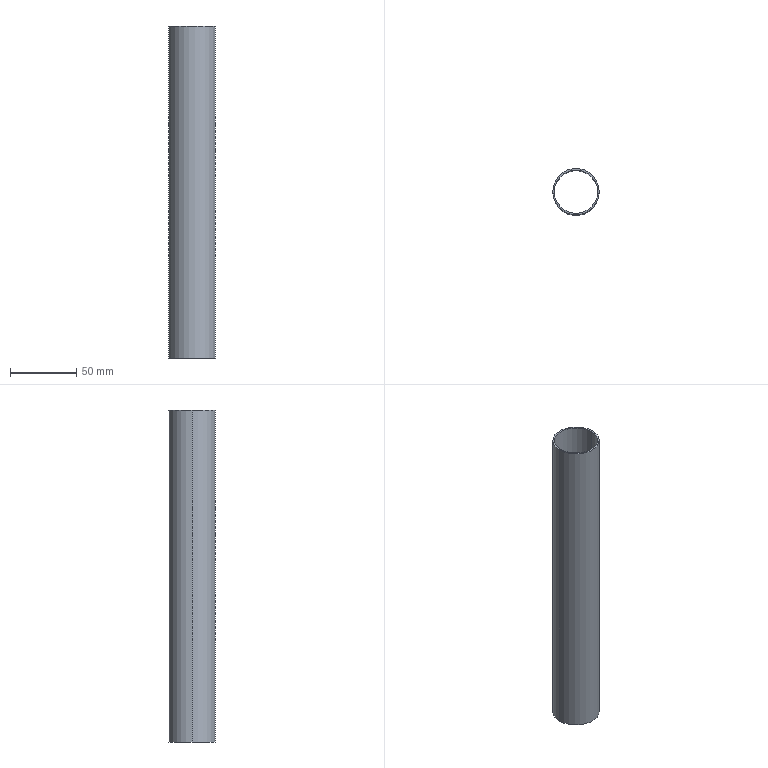Part | STEP file | copper tube 41 | 1 solid | 6 faces | box 35 x 35 x 250 mm | volume 31856 mm3 | cylinder 4 | plane 2 | commonest cylinder face diameters 32.6 x2 35 x2
STEP:
#1=CARTESIAN_POINT('',(0.,0.,0.));
#2=DIRECTION('',(0.,0.,1.));
#3=DIRECTION('',(1.,0.,0.));
#4=AXIS2_PLACEMENT_3D('',#1,#2,#3);
#5=CARTESIAN_POINT('',(16.3,0.,-5.));
#6=VERTEX_POINT('',#5);
#7=CARTESIAN_POINT('',(16.3,0.,245.));
#8=VERTEX_POINT('',#7);
#9=CARTESIAN_POINT('',(16.3,0.,-5.));
#10=DIRECTION('',(0.,0.,1.));
#11=VECTOR('',#10,1.);
#12=LINE('',#9,#11);
#13=CARTESIAN_POINT('',(0.,0.,-5.));
#14=DIRECTION('',(0.,0.,1.));
#15=DIRECTION('',(1.,0.,0.));
#16=AXIS2_PLACEMENT_3D('',#13,#14,#15);
#17=CYLINDRICAL_SURFACE('',#16,16.3);
#18=CARTESIAN_POINT('',(6.283,0.));
#19=DIRECTION('',(0.,1.));
#20=VECTOR('',#19,1.);
#21=LINE('',#18,#20);
#22=(GEOMETRIC_REPRESENTATION_CONTEXT(2)PARAMETRIC_REPRESENTATION_CONTEXT()REPRESENTATION_CONTEXT('',''));
#23=DEFINITIONAL_REPRESENTATION('',(#21),#22);
#24=PCURVE('',#17,#23);
#25=CARTESIAN_POINT('',(0.,0.,-5.));
#26=DIRECTION('',(0.,0.,1.));
#27=DIRECTION('',(1.,0.,0.));
#28=AXIS2_PLACEMENT_3D('',#25,#26,#27);
#29=CYLINDRICAL_SURFACE('',#28,16.3);
#30=CARTESIAN_POINT('',(0.,0.));
#31=DIRECTION('',(0.,1.));
#32=VECTOR('',#31,1.);
#33=LINE('',#30,#32);
#34=(GEOMETRIC_REPRESENTATION_CONTEXT(2)PARAMETRIC_REPRESENTATION_CONTEXT()REPRESENTATION_CONTEXT('',''));
#35=DEFINITIONAL_REPRESENTATION('',(#33),#34);
#36=PCURVE('',#29,#35);
#37=SURFACE_CURVE('',#12,(#24,#36),.PCURVE_S1.);
#38=EDGE_CURVE('',#6,#8,#37,.T.);
#39=ORIENTED_EDGE('',*,*,#38,.T.);
#40=CARTESIAN_POINT('',(-16.3,0.,245.));
#41=VERTEX_POINT('',#40);
#42=CARTESIAN_POINT('',(0.,0.,245.));
#43=DIRECTION('',(0.,0.,1.));
#44=DIRECTION('',(1.,0.,0.));
#45=AXIS2_PLACEMENT_3D('',#42,#43,#44);
#46=CIRCLE('',#45,16.3);
#47=CARTESIAN_POINT('',(0.,250.));
#48=DIRECTION('',(1.,0.));
#49=VECTOR('',#48,1.);
#50=LINE('',#47,#49);
#51=(GEOMETRIC_REPRESENTATION_CONTEXT(2)PARAMETRIC_REPRESENTATION_CONTEXT()REPRESENTATION_CONTEXT('',''));
#52=DEFINITIONAL_REPRESENTATION('',(#50),#51);
#53=PCURVE('',#17,#52);
#54=CARTESIAN_POINT('',(0.,0.,245.));
#55=DIRECTION('',(0.,0.,1.));
#56=DIRECTION('',(1.,0.,0.));
#57=AXIS2_PLACEMENT_3D('',#54,#55,#56);
#58=PLANE('',#57);
#59=CARTESIAN_POINT('',(0.,0.));
#60=DIRECTION('',(1.,0.));
#61=AXIS2_PLACEMENT_2D('',#59,#60);
#62=CIRCLE('',#61,16.3);
#63=(GEOMETRIC_REPRESENTATION_CONTEXT(2)PARAMETRIC_REPRESENTATION_CONTEXT()REPRESENTATION_CONTEXT('',''));
#64=DEFINITIONAL_REPRESENTATION('',(#62),#63);
#65=PCURVE('',#58,#64);
#66=SURFACE_CURVE('',#46,(#53,#65),.PCURVE_S1.);
#67=EDGE_CURVE('',#41,#8,#66,.T.);
#68=ORIENTED_EDGE('',*,*,#67,.F.);
#69=CARTESIAN_POINT('',(-16.3,0.,-5.));
#70=VERTEX_POINT('',#69);
#71=CARTESIAN_POINT('',(-16.3,0.,-5.));
#72=DIRECTION('',(0.,0.,1.));
#73=VECTOR('',#72,1.);
#74=LINE('',#71,#73);
#75=CARTESIAN_POINT('',(3.142,0.));
#76=DIRECTION('',(0.,1.));
#77=VECTOR('',#76,1.);
#78=LINE('',#75,#77);
#79=(GEOMETRIC_REPRESENTATION_CONTEXT(2)PARAMETRIC_REPRESENTATION_CONTEXT()REPRESENTATION_CONTEXT('',''));
#80=DEFINITIONAL_REPRESENTATION('',(#78),#79);
#81=PCURVE('',#17,#80);
#82=CARTESIAN_POINT('',(3.142,0.));
#83=DIRECTION('',(0.,1.));
#84=VECTOR('',#83,1.);
#85=LINE('',#82,#84);
#86=(GEOMETRIC_REPRESENTATION_CONTEXT(2)PARAMETRIC_REPRESENTATION_CONTEXT()REPRESENTATION_CONTEXT('',''));
#87=DEFINITIONAL_REPRESENTATION('',(#85),#86);
#88=PCURVE('',#29,#87);
#89=SURFACE_CURVE('',#74,(#81,#88),.PCURVE_S1.);
#90=EDGE_CURVE('',#70,#41,#89,.T.);
#91=ORIENTED_EDGE('',*,*,#90,.F.);
#92=CARTESIAN_POINT('',(0.,0.,-5.));
#93=DIRECTION('',(0.,0.,1.));
#94=DIRECTION('',(1.,0.,0.));
#95=AXIS2_PLACEMENT_3D('',#92,#93,#94);
#96=CIRCLE('',#95,16.3);
#97=CARTESIAN_POINT('',(0.,0.));
#98=DIRECTION('',(1.,0.));
#99=VECTOR('',#98,1.);
#100=LINE('',#97,#99);
#101=(GEOMETRIC_REPRESENTATION_CONTEXT(2)PARAMETRIC_REPRESENTATION_CONTEXT()REPRESENTATION_CONTEXT('',''));
#102=DEFINITIONAL_REPRESENTATION('',(#100),#101);
#103=PCURVE('',#17,#102);
#104=CARTESIAN_POINT('',(0.,0.,-5.));
#105=DIRECTION('',(0.,0.,1.));
#106=DIRECTION('',(1.,0.,0.));
#107=AXIS2_PLACEMENT_3D('',#104,#105,#106);
#108=PLANE('',#107);
#109=CARTESIAN_POINT('',(0.,0.));
#110=DIRECTION('',(1.,0.));
#111=AXIS2_PLACEMENT_2D('',#109,#110);
#112=CIRCLE('',#111,16.3);
#113=(GEOMETRIC_REPRESENTATION_CONTEXT(2)PARAMETRIC_REPRESENTATION_CONTEXT()REPRESENTATION_CONTEXT('',''));
#114=DEFINITIONAL_REPRESENTATION('',(#112),#113);
#115=PCURVE('',#108,#114);
#116=SURFACE_CURVE('',#96,(#103,#115),.PCURVE_S1.);
#117=EDGE_CURVE('',#70,#6,#116,.T.);
#118=ORIENTED_EDGE('',*,*,#117,.T.);
#119=EDGE_LOOP('',(#39,#68,#91,#118));
#120=FACE_BOUND('',#119,.F.);
#121=ADVANCED_FACE('',(#120),#17,.F.);
#122=CARTESIAN_POINT('',(17.5,0.,245.));
#123=VERTEX_POINT('',#122);
#124=CARTESIAN_POINT('',(-17.5,0.,245.));
#125=VERTEX_POINT('',#124);
#126=CARTESIAN_POINT('',(0.,0.,245.));
#127=DIRECTION('',(0.,0.,1.));
#128=DIRECTION('',(1.,0.,0.));
#129=AXIS2_PLACEMENT_3D('',#126,#127,#128);
#130=CIRCLE('',#129,17.5);
#131=CARTESIAN_POINT('',(0.,0.,245.));
#132=DIRECTION('',(0.,0.,-1.));
#133=DIRECTION('',(-1.,0.,0.));
#134=AXIS2_PLACEMENT_3D('',#131,#132,#133);
#135=CYLINDRICAL_SURFACE('',#134,17.5);
#136=CARTESIAN_POINT('',(3.142,0.));
#137=DIRECTION('',(-1.,0.));
#138=VECTOR('',#137,1.);
#139=LINE('',#136,#138);
#140=(GEOMETRIC_REPRESENTATION_CONTEXT(2)PARAMETRIC_REPRESENTATION_CONTEXT()REPRESENTATION_CONTEXT('',''));
#141=DEFINITIONAL_REPRESENTATION('',(#139),#140);
#142=PCURVE('',#135,#141);
#143=CARTESIAN_POINT('',(0.,0.));
#144=DIRECTION('',(1.,0.));
#145=AXIS2_PLACEMENT_2D('',#143,#144);
#146=CIRCLE('',#145,17.5);
#147=(GEOMETRIC_REPRESENTATION_CONTEXT(2)PARAMETRIC_REPRESENTATION_CONTEXT()REPRESENTATION_CONTEXT('',''));
#148=DEFINITIONAL_REPRESENTATION('',(#146),#147);
#149=PCURVE('',#58,#148);
#150=SURFACE_CURVE('',#130,(#142,#149),.PCURVE_S1.);
#151=EDGE_CURVE('',#123,#125,#150,.T.);
#152=ORIENTED_EDGE('',*,*,#151,.F.);
#153=CARTESIAN_POINT('',(17.5,0.,-5.));
#154=VERTEX_POINT('',#153);
#155=CARTESIAN_POINT('',(17.5,0.,245.));
#156=DIRECTION('',(0.,0.,-1.));
#157=VECTOR('',#156,1.);
#158=LINE('',#155,#157);
#159=CARTESIAN_POINT('',(3.142,0.));
#160=DIRECTION('',(0.,1.));
#161=VECTOR('',#160,1.);
#162=LINE('',#159,#161);
#163=(GEOMETRIC_REPRESENTATION_CONTEXT(2)PARAMETRIC_REPRESENTATION_CONTEXT()REPRESENTATION_CONTEXT('',''));
#164=DEFINITIONAL_REPRESENTATION('',(#162),#163);
#165=PCURVE('',#135,#164);
#166=CARTESIAN_POINT('',(0.,0.,245.));
#167=DIRECTION('',(0.,0.,-1.));
#168=DIRECTION('',(-1.,0.,0.));
#169=AXIS2_PLACEMENT_3D('',#166,#167,#168);
#170=CYLINDRICAL_SURFACE('',#169,17.5);
#171=CARTESIAN_POINT('',(3.142,0.));
#172=DIRECTION('',(0.,1.));
#173=VECTOR('',#172,1.);
#174=LINE('',#171,#173);
#175=(GEOMETRIC_REPRESENTATION_CONTEXT(2)PARAMETRIC_REPRESENTATION_CONTEXT()REPRESENTATION_CONTEXT('',''));
#176=DEFINITIONAL_REPRESENTATION('',(#174),#175);
#177=PCURVE('',#170,#176);
#178=SURFACE_CURVE('',#158,(#165,#177),.PCURVE_S1.);
#179=EDGE_CURVE('',#123,#154,#178,.T.);
#180=ORIENTED_EDGE('',*,*,#179,.T.);
#181=CARTESIAN_POINT('',(-17.5,0.,-5.));
#182=VERTEX_POINT('',#181);
#183=CARTESIAN_POINT('',(0.,0.,-5.));
#184=DIRECTION('',(0.,0.,1.));
#185=DIRECTION('',(1.,0.,0.));
#186=AXIS2_PLACEMENT_3D('',#183,#184,#185);
#187=CIRCLE('',#186,17.5);
#188=CARTESIAN_POINT('',(3.142,250.));
#189=DIRECTION('',(-1.,0.));
#190=VECTOR('',#189,1.);
#191=LINE('',#188,#190);
#192=(GEOMETRIC_REPRESENTATION_CONTEXT(2)PARAMETRIC_REPRESENTATION_CONTEXT()REPRESENTATION_CONTEXT('',''));
#193=DEFINITIONAL_REPRESENTATION('',(#191),#192);
#194=PCURVE('',#135,#193);
#195=CARTESIAN_POINT('',(0.,0.));
#196=DIRECTION('',(1.,0.));
#197=AXIS2_PLACEMENT_2D('',#195,#196);
#198=CIRCLE('',#197,17.5);
#199=(GEOMETRIC_REPRESENTATION_CONTEXT(2)PARAMETRIC_REPRESENTATION_CONTEXT()REPRESENTATION_CONTEXT('',''));
#200=DEFINITIONAL_REPRESENTATION('',(#198),#199);
#201=PCURVE('',#108,#200);
#202=SURFACE_CURVE('',#187,(#194,#201),.PCURVE_S1.);
#203=EDGE_CURVE('',#154,#182,#202,.T.);
#204=ORIENTED_EDGE('',*,*,#203,.T.);
#205=CARTESIAN_POINT('',(-17.5,0.,245.));
#206=DIRECTION('',(0.,0.,-1.));
#207=VECTOR('',#206,1.);
#208=LINE('',#205,#207);
#209=CARTESIAN_POINT('',(0.,0.));
#210=DIRECTION('',(0.,1.));
#211=VECTOR('',#210,1.);
#212=LINE('',#209,#211);
#213=(GEOMETRIC_REPRESENTATION_CONTEXT(2)PARAMETRIC_REPRESENTATION_CONTEXT()REPRESENTATION_CONTEXT('',''));
#214=DEFINITIONAL_REPRESENTATION('',(#212),#213);
#215=PCURVE('',#135,#214);
#216=CARTESIAN_POINT('',(6.283,0.));
#217=DIRECTION('',(0.,1.));
#218=VECTOR('',#217,1.);
#219=LINE('',#216,#218);
#220=(GEOMETRIC_REPRESENTATION_CONTEXT(2)PARAMETRIC_REPRESENTATION_CONTEXT()REPRESENTATION_CONTEXT('',''));
#221=DEFINITIONAL_REPRESENTATION('',(#219),#220);
#222=PCURVE('',#170,#221);
#223=SURFACE_CURVE('',#208,(#215,#222),.PCURVE_S1.);
#224=EDGE_CURVE('',#125,#182,#223,.T.);
#225=ORIENTED_EDGE('',*,*,#224,.F.);
#226=EDGE_LOOP('',(#152,#180,#204,#225));
#227=FACE_BOUND('',#226,.T.);
#228=ADVANCED_FACE('',(#227),#135,.T.);
#229=ORIENTED_EDGE('',*,*,#179,.F.);
#230=CARTESIAN_POINT('',(0.,0.,245.));
#231=DIRECTION('',(0.,0.,1.));
#232=DIRECTION('',(1.,0.,0.));
#233=AXIS2_PLACEMENT_3D('',#230,#231,#232);
#234=CIRCLE('',#233,17.5);
#235=CARTESIAN_POINT('',(9.425,0.));
#236=DIRECTION('',(-1.,0.));
#237=VECTOR('',#236,1.);
#238=LINE('',#235,#237);
#239=(GEOMETRIC_REPRESENTATION_CONTEXT(2)PARAMETRIC_REPRESENTATION_CONTEXT()REPRESENTATION_CONTEXT('',''));
#240=DEFINITIONAL_REPRESENTATION('',(#238),#239);
#241=PCURVE('',#170,#240);
#242=CARTESIAN_POINT('',(0.,0.));
#243=DIRECTION('',(1.,0.));
#244=AXIS2_PLACEMENT_2D('',#242,#243);
#245=CIRCLE('',#244,17.5);
#246=(GEOMETRIC_REPRESENTATION_CONTEXT(2)PARAMETRIC_REPRESENTATION_CONTEXT()REPRESENTATION_CONTEXT('',''));
#247=DEFINITIONAL_REPRESENTATION('',(#245),#246);
#248=PCURVE('',#58,#247);
#249=SURFACE_CURVE('',#234,(#241,#248),.PCURVE_S1.);
#250=EDGE_CURVE('',#125,#123,#249,.T.);
#251=ORIENTED_EDGE('',*,*,#250,.F.);
#252=ORIENTED_EDGE('',*,*,#224,.T.);
#253=CARTESIAN_POINT('',(0.,0.,-5.));
#254=DIRECTION('',(0.,0.,1.));
#255=DIRECTION('',(1.,0.,0.));
#256=AXIS2_PLACEMENT_3D('',#253,#254,#255);
#257=CIRCLE('',#256,17.5);
#258=CARTESIAN_POINT('',(9.425,250.));
#259=DIRECTION('',(-1.,0.));
#260=VECTOR('',#259,1.);
#261=LINE('',#258,#260);
#262=(GEOMETRIC_REPRESENTATION_CONTEXT(2)PARAMETRIC_REPRESENTATION_CONTEXT()REPRESENTATION_CONTEXT('',''));
#263=DEFINITIONAL_REPRESENTATION('',(#261),#262);
#264=PCURVE('',#170,#263);
#265=CARTESIAN_POINT('',(0.,0.));
#266=DIRECTION('',(1.,0.));
#267=AXIS2_PLACEMENT_2D('',#265,#266);
#268=CIRCLE('',#267,17.5);
#269=(GEOMETRIC_REPRESENTATION_CONTEXT(2)PARAMETRIC_REPRESENTATION_CONTEXT()REPRESENTATION_CONTEXT('',''));
#270=DEFINITIONAL_REPRESENTATION('',(#268),#269);
#271=PCURVE('',#108,#270);
#272=SURFACE_CURVE('',#257,(#264,#271),.PCURVE_S1.);
#273=EDGE_CURVE('',#182,#154,#272,.T.);
#274=ORIENTED_EDGE('',*,*,#273,.T.);
#275=EDGE_LOOP('',(#229,#251,#252,#274));
#276=FACE_BOUND('',#275,.T.);
#277=ADVANCED_FACE('',(#276),#170,.T.);
#278=CARTESIAN_POINT('',(0.,0.,245.));
#279=DIRECTION('',(0.,0.,1.));
#280=DIRECTION('',(1.,0.,0.));
#281=AXIS2_PLACEMENT_3D('',#278,#279,#280);
#282=CIRCLE('',#281,16.3);
#283=CARTESIAN_POINT('',(0.,0.));
#284=DIRECTION('',(1.,0.));
#285=AXIS2_PLACEMENT_2D('',#283,#284);
#286=CIRCLE('',#285,16.3);
#287=(GEOMETRIC_REPRESENTATION_CONTEXT(2)PARAMETRIC_REPRESENTATION_CONTEXT()REPRESENTATION_CONTEXT('',''));
#288=DEFINITIONAL_REPRESENTATION('',(#286),#287);
#289=PCURVE('',#58,#288);
#290=CARTESIAN_POINT('',(0.,250.));
#291=DIRECTION('',(1.,0.));
#292=VECTOR('',#291,1.);
#293=LINE('',#290,#292);
#294=(GEOMETRIC_REPRESENTATION_CONTEXT(2)PARAMETRIC_REPRESENTATION_CONTEXT()REPRESENTATION_CONTEXT('',''));
#295=DEFINITIONAL_REPRESENTATION('',(#293),#294);
#296=PCURVE('',#29,#295);
#297=SURFACE_CURVE('',#282,(#289,#296),.PCURVE_S1.);
#298=EDGE_CURVE('',#8,#41,#297,.T.);
#299=ORIENTED_EDGE('',*,*,#298,.F.);
#300=ORIENTED_EDGE('',*,*,#67,.F.);
#301=EDGE_LOOP('',(#299,#300));
#302=FACE_BOUND('',#301,.T.);
#303=ORIENTED_EDGE('',*,*,#250,.T.);
#304=ORIENTED_EDGE('',*,*,#151,.T.);
#305=EDGE_LOOP('',(#303,#304));
#306=FACE_BOUND('',#305,.T.);
#307=ADVANCED_FACE('',(#302,#306),#58,.T.);
#308=CARTESIAN_POINT('',(0.,0.,-5.));
#309=DIRECTION('',(0.,0.,1.));
#310=DIRECTION('',(1.,0.,0.));
#311=AXIS2_PLACEMENT_3D('',#308,#309,#310);
#312=CIRCLE('',#311,16.3);
#313=CARTESIAN_POINT('',(0.,0.));
#314=DIRECTION('',(1.,0.));
#315=AXIS2_PLACEMENT_2D('',#313,#314);
#316=CIRCLE('',#315,16.3);
#317=(GEOMETRIC_REPRESENTATION_CONTEXT(2)PARAMETRIC_REPRESENTATION_CONTEXT()REPRESENTATION_CONTEXT('',''));
#318=DEFINITIONAL_REPRESENTATION('',(#316),#317);
#319=PCURVE('',#108,#318);
#320=CARTESIAN_POINT('',(0.,0.));
#321=DIRECTION('',(1.,0.));
#322=VECTOR('',#321,1.);
#323=LINE('',#320,#322);
#324=(GEOMETRIC_REPRESENTATION_CONTEXT(2)PARAMETRIC_REPRESENTATION_CONTEXT()REPRESENTATION_CONTEXT('',''));
#325=DEFINITIONAL_REPRESENTATION('',(#323),#324);
#326=PCURVE('',#29,#325);
#327=SURFACE_CURVE('',#312,(#319,#326),.PCURVE_S1.);
#328=EDGE_CURVE('',#6,#70,#327,.T.);
#329=ORIENTED_EDGE('',*,*,#328,.T.);
#330=ORIENTED_EDGE('',*,*,#117,.T.);
#331=EDGE_LOOP('',(#329,#330));
#332=FACE_BOUND('',#331,.T.);
#333=ORIENTED_EDGE('',*,*,#273,.F.);
#334=ORIENTED_EDGE('',*,*,#203,.F.);
#335=EDGE_LOOP('',(#333,#334));
#336=FACE_BOUND('',#335,.T.);
#337=ADVANCED_FACE('',(#332,#336),#108,.F.);
#338=ORIENTED_EDGE('',*,*,#298,.F.);
#339=ORIENTED_EDGE('',*,*,#38,.F.);
#340=ORIENTED_EDGE('',*,*,#328,.T.);
#341=ORIENTED_EDGE('',*,*,#90,.T.);
#342=EDGE_LOOP('',(#338,#339,#340,#341));
#343=FACE_BOUND('',#342,.F.);
#344=ADVANCED_FACE('',(#343),#29,.F.);
#345=CLOSED_SHELL('',(#121,#228,#277,#307,#337,#344));
#346=MANIFOLD_SOLID_BREP('',#345);
#347=(LENGTH_UNIT()NAMED_UNIT(*)SI_UNIT(.MILLI.,.METRE.));
#348=UNCERTAINTY_MEASURE_WITH_UNIT(LENGTH_MEASURE(0.0000001),#347,'','');
#349=(NAMED_UNIT(*)PLANE_ANGLE_UNIT()SI_UNIT($,.RADIAN.));
#350=(NAMED_UNIT(*)SI_UNIT($,.STERADIAN.)SOLID_ANGLE_UNIT());
#351=(GEOMETRIC_REPRESENTATION_CONTEXT(3)GLOBAL_UNCERTAINTY_ASSIGNED_CONTEXT((#348))GLOBAL_UNIT_ASSIGNED_CONTEXT((#347,#349,#350))REPRESENTATION_CONTEXT('',''));
#352=ADVANCED_BREP_SHAPE_REPRESENTATION('',(#4,#346),#351);